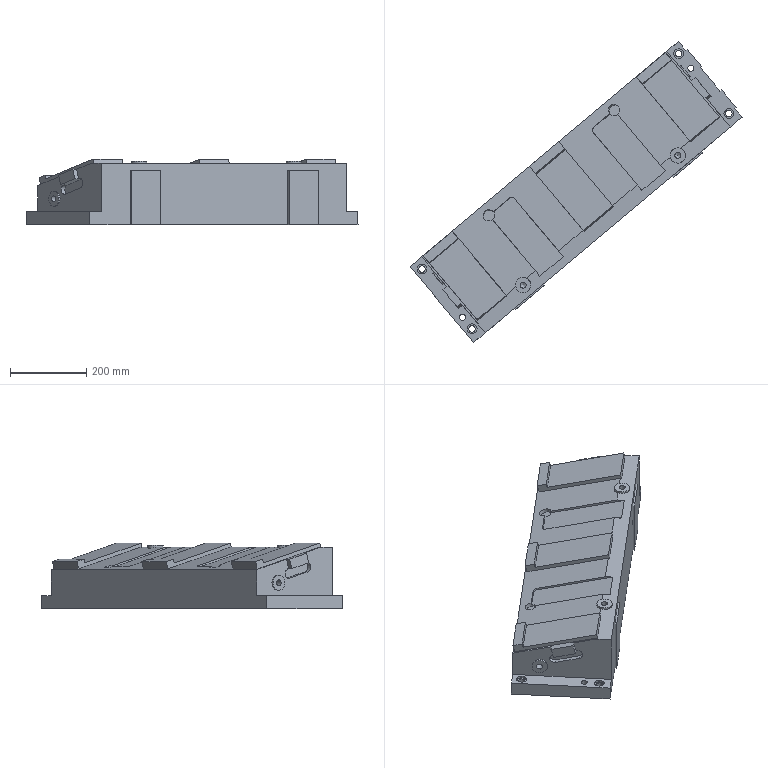Part | NX | features solid 2 | 1 solid | 128 faces | box 871.886 x 790.536 x 172.478 mm | volume 22389263 mm3 | plane 97 | cylinder 26 | cone 4 | spline 1 | commonest cylinder face diameters 16 x6 17 x4 25 x4 26 x4 40 x4 20 x2